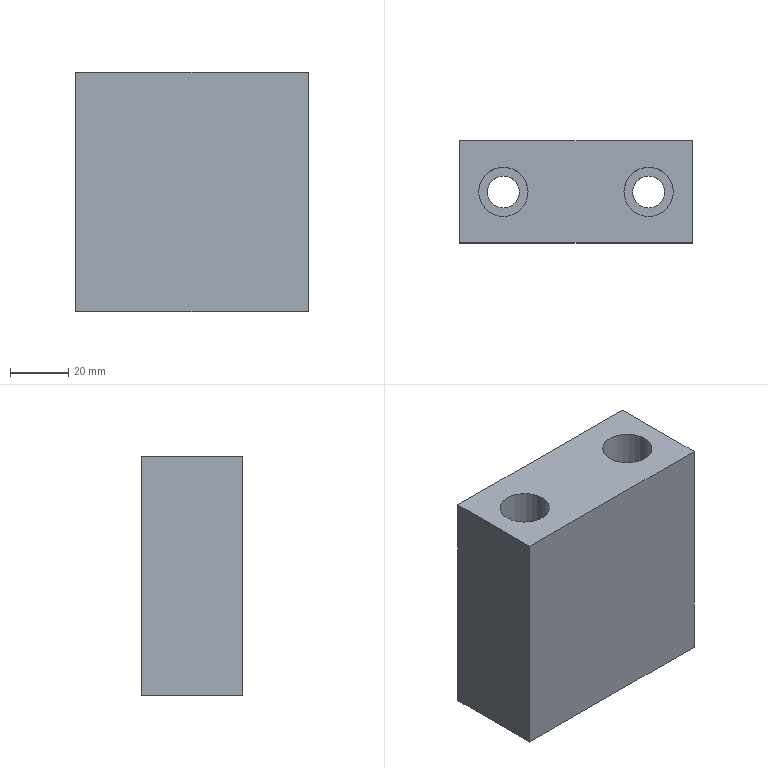Part | STEP file | lll_id4294_x_t | 1 solid | 12 faces | box 80 x 35 x 82.5 mm | volume 201465 mm3 | plane 8 | cylinder 4 | commonest cylinder face diameters 11 x2 17 x2
STEP:
#1=CARTESIAN_POINT('',(3404.435,362.,2.5));
#2=VERTEX_POINT('',#1);
#3=CARTESIAN_POINT('',(3324.435,362.,2.5));
#4=VERTEX_POINT('',#3);
#5=CARTESIAN_POINT('',(3354.435,362.,2.5));
#6=DIRECTION('',(-1.,0.,0.));
#7=VECTOR('',#6,1.);
#8=LINE('',#5,#7);
#9=EDGE_CURVE('',#2,#4,#8,.T.);
#10=ORIENTED_EDGE('',*,*,#9,.T.);
#11=CARTESIAN_POINT('',(3324.435,327.,2.5));
#12=VERTEX_POINT('',#11);
#13=CARTESIAN_POINT('',(3324.435,342.,2.5));
#14=DIRECTION('',(0.,-1.,0.));
#15=VECTOR('',#14,1.);
#16=LINE('',#13,#15);
#17=EDGE_CURVE('',#4,#12,#16,.T.);
#18=ORIENTED_EDGE('',*,*,#17,.T.);
#19=CARTESIAN_POINT('',(3404.435,327.,2.5));
#20=VERTEX_POINT('',#19);
#21=CARTESIAN_POINT('',(3354.435,327.,2.5));
#22=DIRECTION('',(1.,0.,0.));
#23=VECTOR('',#22,1.);
#24=LINE('',#21,#23);
#25=EDGE_CURVE('',#12,#20,#24,.T.);
#26=ORIENTED_EDGE('',*,*,#25,.T.);
#27=CARTESIAN_POINT('',(3404.435,342.,2.5));
#28=DIRECTION('',(0.,1.,0.));
#29=VECTOR('',#28,1.);
#30=LINE('',#27,#29);
#31=EDGE_CURVE('',#20,#2,#30,.T.);
#32=ORIENTED_EDGE('',*,*,#31,.T.);
#33=EDGE_LOOP('',(#10,#18,#26,#32));
#34=FACE_BOUND('',#33,.T.);
#35=CARTESIAN_POINT('',(3330.935,344.5,2.5));
#36=VERTEX_POINT('',#35);
#37=CARTESIAN_POINT('',(3339.435,344.5,2.5));
#38=DIRECTION('',(0.,0.,-1.));
#39=DIRECTION('',(-1.,0.,0.));
#40=AXIS2_PLACEMENT_3D('',#37,#38,#39);
#41=CIRCLE('',#40,8.5);
#42=EDGE_CURVE('',#36,#36,#41,.T.);
#43=ORIENTED_EDGE('',*,*,#42,.T.);
#44=EDGE_LOOP('',(#43));
#45=FACE_BOUND('',#44,.T.);
#46=CARTESIAN_POINT('',(3380.935,344.5,2.5));
#47=VERTEX_POINT('',#46);
#48=CARTESIAN_POINT('',(3389.435,344.5,2.5));
#49=DIRECTION('',(0.,0.,1.));
#50=DIRECTION('',(-1.,0.,0.));
#51=AXIS2_PLACEMENT_3D('',#48,#49,#50);
#52=CIRCLE('',#51,8.5);
#53=EDGE_CURVE('',#47,#47,#52,.T.);
#54=ORIENTED_EDGE('',*,*,#53,.F.);
#55=EDGE_LOOP('',(#54));
#56=FACE_BOUND('',#55,.T.);
#57=CARTESIAN_POINT('',(5309.435,-238.,2.5));
#58=DIRECTION('',(0.,0.,-1.));
#59=DIRECTION('',(-1.,0.,0.));
#60=AXIS2_PLACEMENT_3D('',#57,#58,#59);
#61=PLANE('',#60);
#62=ADVANCED_FACE('',(#34,#45,#56),#61,.F.);
#63=CARTESIAN_POINT('',(3394.935,344.5,-80.));
#64=VERTEX_POINT('',#63);
#65=CARTESIAN_POINT('',(3389.435,344.5,-80.));
#66=DIRECTION('',(0.,0.,1.));
#67=DIRECTION('',(1.,0.,0.));
#68=AXIS2_PLACEMENT_3D('',#65,#66,#67);
#69=CIRCLE('',#68,5.5);
#70=EDGE_CURVE('',#64,#64,#69,.T.);
#71=ORIENTED_EDGE('',*,*,#70,.T.);
#72=EDGE_LOOP('',(#71));
#73=FACE_BOUND('',#72,.T.);
#74=CARTESIAN_POINT('',(3404.435,362.,-80.));
#75=VERTEX_POINT('',#74);
#76=CARTESIAN_POINT('',(3404.435,327.,-80.));
#77=VERTEX_POINT('',#76);
#78=CARTESIAN_POINT('',(3404.435,342.,-80.));
#79=DIRECTION('',(0.,-1.,0.));
#80=VECTOR('',#79,1.);
#81=LINE('',#78,#80);
#82=EDGE_CURVE('',#75,#77,#81,.T.);
#83=ORIENTED_EDGE('',*,*,#82,.T.);
#84=CARTESIAN_POINT('',(3324.435,327.,-80.));
#85=VERTEX_POINT('',#84);
#86=CARTESIAN_POINT('',(3354.435,327.,-80.));
#87=DIRECTION('',(-1.,0.,0.));
#88=VECTOR('',#87,1.);
#89=LINE('',#86,#88);
#90=EDGE_CURVE('',#77,#85,#89,.T.);
#91=ORIENTED_EDGE('',*,*,#90,.T.);
#92=CARTESIAN_POINT('',(3324.435,362.,-80.));
#93=VERTEX_POINT('',#92);
#94=CARTESIAN_POINT('',(3324.435,342.,-80.));
#95=DIRECTION('',(0.,1.,0.));
#96=VECTOR('',#95,1.);
#97=LINE('',#94,#96);
#98=EDGE_CURVE('',#85,#93,#97,.T.);
#99=ORIENTED_EDGE('',*,*,#98,.T.);
#100=CARTESIAN_POINT('',(3354.435,362.,-80.));
#101=DIRECTION('',(1.,0.,0.));
#102=VECTOR('',#101,1.);
#103=LINE('',#100,#102);
#104=EDGE_CURVE('',#93,#75,#103,.T.);
#105=ORIENTED_EDGE('',*,*,#104,.T.);
#106=EDGE_LOOP('',(#83,#91,#99,#105));
#107=FACE_BOUND('',#106,.T.);
#108=CARTESIAN_POINT('',(3333.935,344.5,-80.));
#109=VERTEX_POINT('',#108);
#110=CARTESIAN_POINT('',(3339.435,344.5,-80.));
#111=DIRECTION('',(0.,0.,-1.));
#112=DIRECTION('',(-1.,0.,0.));
#113=AXIS2_PLACEMENT_3D('',#110,#111,#112);
#114=CIRCLE('',#113,5.5);
#115=EDGE_CURVE('',#109,#109,#114,.T.);
#116=ORIENTED_EDGE('',*,*,#115,.F.);
#117=EDGE_LOOP('',(#116));
#118=FACE_BOUND('',#117,.T.);
#119=CARTESIAN_POINT('',(3354.435,342.,-80.));
#120=DIRECTION('',(0.,0.,-1.));
#121=DIRECTION('',(-1.,0.,0.));
#122=AXIS2_PLACEMENT_3D('',#119,#120,#121);
#123=PLANE('',#122);
#124=ADVANCED_FACE('',(#73,#107,#118),#123,.T.);
#125=CARTESIAN_POINT('',(3404.435,362.,-80.));
#126=DIRECTION('',(0.,0.,1.));
#127=VECTOR('',#126,1.);
#128=LINE('',#125,#127);
#129=EDGE_CURVE('',#75,#2,#128,.T.);
#130=ORIENTED_EDGE('',*,*,#129,.F.);
#131=ORIENTED_EDGE('',*,*,#104,.F.);
#132=CARTESIAN_POINT('',(3324.435,362.,-80.));
#133=DIRECTION('',(0.,0.,1.));
#134=VECTOR('',#133,1.);
#135=LINE('',#132,#134);
#136=EDGE_CURVE('',#93,#4,#135,.T.);
#137=ORIENTED_EDGE('',*,*,#136,.T.);
#138=ORIENTED_EDGE('',*,*,#9,.F.);
#139=EDGE_LOOP('',(#130,#131,#137,#138));
#140=FACE_OUTER_BOUND('',#139,.T.);
#141=CARTESIAN_POINT('',(3354.435,362.,-80.));
#142=DIRECTION('',(0.,1.,0.));
#143=DIRECTION('',(0.,0.,-1.));
#144=AXIS2_PLACEMENT_3D('',#141,#142,#143);
#145=PLANE('',#144);
#146=ADVANCED_FACE('',(#140),#145,.T.);
#147=ORIENTED_EDGE('',*,*,#136,.F.);
#148=ORIENTED_EDGE('',*,*,#98,.F.);
#149=CARTESIAN_POINT('',(3324.435,327.,-80.));
#150=DIRECTION('',(0.,0.,1.));
#151=VECTOR('',#150,1.);
#152=LINE('',#149,#151);
#153=EDGE_CURVE('',#85,#12,#152,.T.);
#154=ORIENTED_EDGE('',*,*,#153,.T.);
#155=ORIENTED_EDGE('',*,*,#17,.F.);
#156=EDGE_LOOP('',(#147,#148,#154,#155));
#157=FACE_OUTER_BOUND('',#156,.T.);
#158=CARTESIAN_POINT('',(3324.435,342.,-80.));
#159=DIRECTION('',(-1.,0.,0.));
#160=DIRECTION('',(0.,0.,1.));
#161=AXIS2_PLACEMENT_3D('',#158,#159,#160);
#162=PLANE('',#161);
#163=ADVANCED_FACE('',(#157),#162,.T.);
#164=ORIENTED_EDGE('',*,*,#153,.F.);
#165=ORIENTED_EDGE('',*,*,#90,.F.);
#166=CARTESIAN_POINT('',(3404.435,327.,-80.));
#167=DIRECTION('',(0.,0.,1.));
#168=VECTOR('',#167,1.);
#169=LINE('',#166,#168);
#170=EDGE_CURVE('',#77,#20,#169,.T.);
#171=ORIENTED_EDGE('',*,*,#170,.T.);
#172=ORIENTED_EDGE('',*,*,#25,.F.);
#173=EDGE_LOOP('',(#164,#165,#171,#172));
#174=FACE_OUTER_BOUND('',#173,.T.);
#175=CARTESIAN_POINT('',(3354.435,327.,-80.));
#176=DIRECTION('',(0.,-1.,0.));
#177=DIRECTION('',(0.,0.,1.));
#178=AXIS2_PLACEMENT_3D('',#175,#176,#177);
#179=PLANE('',#178);
#180=ADVANCED_FACE('',(#174),#179,.T.);
#181=ORIENTED_EDGE('',*,*,#82,.F.);
#182=ORIENTED_EDGE('',*,*,#129,.T.);
#183=ORIENTED_EDGE('',*,*,#31,.F.);
#184=ORIENTED_EDGE('',*,*,#170,.F.);
#185=EDGE_LOOP('',(#181,#182,#183,#184));
#186=FACE_OUTER_BOUND('',#185,.T.);
#187=CARTESIAN_POINT('',(3404.435,342.,-80.));
#188=DIRECTION('',(1.,0.,0.));
#189=DIRECTION('',(0.,0.,-1.));
#190=AXIS2_PLACEMENT_3D('',#187,#188,#189);
#191=PLANE('',#190);
#192=ADVANCED_FACE('',(#186),#191,.T.);
#193=CARTESIAN_POINT('',(3330.935,344.5,-50.));
#194=VERTEX_POINT('',#193);
#195=CARTESIAN_POINT('',(3339.435,344.5,-50.));
#196=DIRECTION('',(0.,0.,1.));
#197=DIRECTION('',(-1.,0.,0.));
#198=AXIS2_PLACEMENT_3D('',#195,#196,#197);
#199=CIRCLE('',#198,8.5);
#200=EDGE_CURVE('',#194,#194,#199,.T.);
#201=ORIENTED_EDGE('',*,*,#200,.F.);
#202=EDGE_LOOP('',(#201));
#203=FACE_BOUND('',#202,.T.);
#204=ORIENTED_EDGE('',*,*,#42,.F.);
#205=EDGE_LOOP('',(#204));
#206=FACE_BOUND('',#205,.T.);
#207=CARTESIAN_POINT('',(3339.435,344.5,3.2));
#208=DIRECTION('',(0.,0.,-1.));
#209=DIRECTION('',(1.,0.,0.));
#210=AXIS2_PLACEMENT_3D('',#207,#208,#209);
#211=CYLINDRICAL_SURFACE('',#210,8.5);
#212=ADVANCED_FACE('',(#203,#206),#211,.F.);
#213=ORIENTED_EDGE('',*,*,#115,.T.);
#214=EDGE_LOOP('',(#213));
#215=FACE_BOUND('',#214,.T.);
#216=CARTESIAN_POINT('',(3333.935,344.5,-50.));
#217=VERTEX_POINT('',#216);
#218=CARTESIAN_POINT('',(3339.435,344.5,-50.));
#219=DIRECTION('',(0.,0.,1.));
#220=DIRECTION('',(-1.,0.,0.));
#221=AXIS2_PLACEMENT_3D('',#218,#219,#220);
#222=CIRCLE('',#221,5.5);
#223=EDGE_CURVE('',#217,#217,#222,.T.);
#224=ORIENTED_EDGE('',*,*,#223,.T.);
#225=EDGE_LOOP('',(#224));
#226=FACE_BOUND('',#225,.T.);
#227=CARTESIAN_POINT('',(3339.435,344.5,-96.8));
#228=DIRECTION('',(0.,0.,-1.));
#229=DIRECTION('',(1.,0.,0.));
#230=AXIS2_PLACEMENT_3D('',#227,#228,#229);
#231=CYLINDRICAL_SURFACE('',#230,5.5);
#232=ADVANCED_FACE('',(#215,#226),#231,.F.);
#233=ORIENTED_EDGE('',*,*,#223,.F.);
#234=EDGE_LOOP('',(#233));
#235=FACE_BOUND('',#234,.T.);
#236=ORIENTED_EDGE('',*,*,#200,.T.);
#237=EDGE_LOOP('',(#236));
#238=FACE_BOUND('',#237,.T.);
#239=CARTESIAN_POINT('',(640.435,-404.5,-50.));
#240=DIRECTION('',(0.,0.,-1.));
#241=DIRECTION('',(-1.,0.,0.));
#242=AXIS2_PLACEMENT_3D('',#239,#240,#241);
#243=PLANE('',#242);
#244=ADVANCED_FACE('',(#235,#238),#243,.F.);
#245=CARTESIAN_POINT('',(3380.935,344.5,-50.));
#246=VERTEX_POINT('',#245);
#247=CARTESIAN_POINT('',(3389.435,344.5,-50.));
#248=DIRECTION('',(0.,0.,-1.));
#249=DIRECTION('',(-1.,0.,0.));
#250=AXIS2_PLACEMENT_3D('',#247,#248,#249);
#251=CIRCLE('',#250,8.5);
#252=EDGE_CURVE('',#246,#246,#251,.T.);
#253=ORIENTED_EDGE('',*,*,#252,.T.);
#254=EDGE_LOOP('',(#253));
#255=FACE_BOUND('',#254,.T.);
#256=ORIENTED_EDGE('',*,*,#53,.T.);
#257=EDGE_LOOP('',(#256));
#258=FACE_BOUND('',#257,.T.);
#259=CARTESIAN_POINT('',(3389.435,344.5,3.2));
#260=DIRECTION('',(0.,0.,-1.));
#261=DIRECTION('',(-1.,0.,0.));
#262=AXIS2_PLACEMENT_3D('',#259,#260,#261);
#263=CYLINDRICAL_SURFACE('',#262,8.5);
#264=ADVANCED_FACE('',(#255,#258),#263,.F.);
#265=ORIENTED_EDGE('',*,*,#70,.F.);
#266=EDGE_LOOP('',(#265));
#267=FACE_BOUND('',#266,.T.);
#268=CARTESIAN_POINT('',(3383.935,344.5,-50.));
#269=VERTEX_POINT('',#268);
#270=CARTESIAN_POINT('',(3389.435,344.5,-50.));
#271=DIRECTION('',(0.,0.,-1.));
#272=DIRECTION('',(-1.,0.,0.));
#273=AXIS2_PLACEMENT_3D('',#270,#271,#272);
#274=CIRCLE('',#273,5.5);
#275=EDGE_CURVE('',#269,#269,#274,.T.);
#276=ORIENTED_EDGE('',*,*,#275,.F.);
#277=EDGE_LOOP('',(#276));
#278=FACE_BOUND('',#277,.T.);
#279=CARTESIAN_POINT('',(3389.435,344.5,-96.8));
#280=DIRECTION('',(0.,0.,-1.));
#281=DIRECTION('',(-1.,0.,0.));
#282=AXIS2_PLACEMENT_3D('',#279,#280,#281);
#283=CYLINDRICAL_SURFACE('',#282,5.5);
#284=ADVANCED_FACE('',(#267,#278),#283,.F.);
#285=ORIENTED_EDGE('',*,*,#275,.T.);
#286=EDGE_LOOP('',(#285));
#287=FACE_BOUND('',#286,.T.);
#288=ORIENTED_EDGE('',*,*,#252,.F.);
#289=EDGE_LOOP('',(#288));
#290=FACE_BOUND('',#289,.T.);
#291=CARTESIAN_POINT('',(640.435,-404.5,-50.));
#292=DIRECTION('',(0.,0.,-1.));
#293=DIRECTION('',(-1.,0.,0.));
#294=AXIS2_PLACEMENT_3D('',#291,#292,#293);
#295=PLANE('',#294);
#296=ADVANCED_FACE('',(#287,#290),#295,.F.);
#297=CLOSED_SHELL('',(#62,#124,#146,#163,#180,#192,#212,#232,#244,#264,#284,#296));
#298=MANIFOLD_SOLID_BREP('',#297);
#299=(LENGTH_UNIT()NAMED_UNIT(*)SI_UNIT(.MILLI.,.METRE.));
#300=UNCERTAINTY_MEASURE_WITH_UNIT(LENGTH_MEASURE(0.00002),#299,'','');
#301=(NAMED_UNIT(*)PLANE_ANGLE_UNIT()SI_UNIT($,.RADIAN.));
#302=PLANE_ANGLE_MEASURE_WITH_UNIT(PLANE_ANGLE_MEASURE(0.01745),#301);
#303=DIMENSIONAL_EXPONENTS(0.,0.,0.,0.,0.,0.,0.);
#304=(CONVERSION_BASED_UNIT('DEGREE',#302)NAMED_UNIT(#303)PLANE_ANGLE_UNIT());
#305=(NAMED_UNIT(*)SI_UNIT($,.STERADIAN.)SOLID_ANGLE_UNIT());
#306=(GEOMETRIC_REPRESENTATION_CONTEXT(3)GLOBAL_UNCERTAINTY_ASSIGNED_CONTEXT((#300))GLOBAL_UNIT_ASSIGNED_CONTEXT((#299,#304,#305))REPRESENTATION_CONTEXT('',''));
#307=ADVANCED_BREP_SHAPE_REPRESENTATION('',(#298),#306);